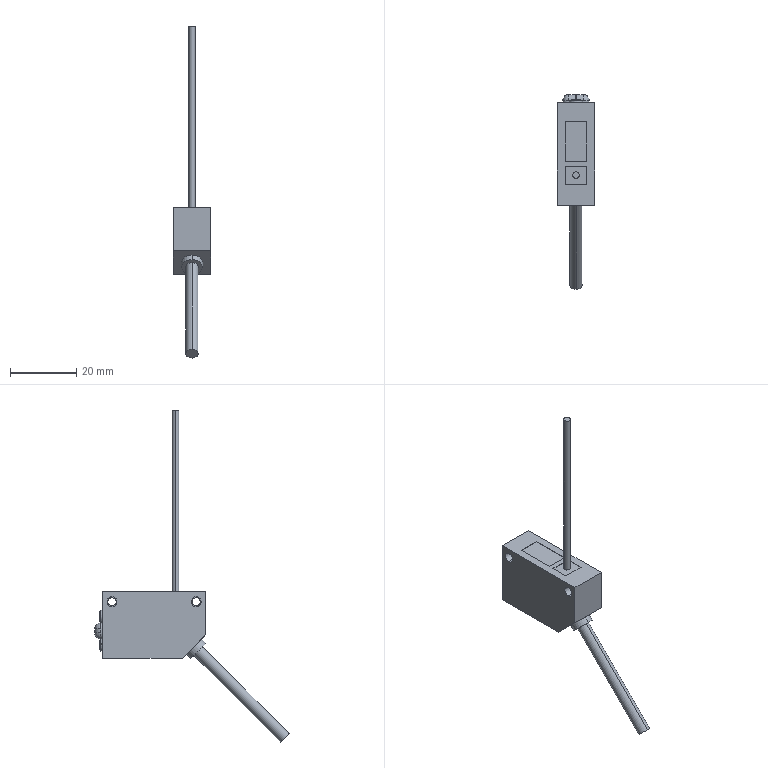Part | STEP file | Compact photoelectric sensor CX-441 | 3 solids | 95 faces | box 11.2 x 58.715 x 100.215 mm | volume 7246 mm3 | plane 50 | cylinder 34 | cone 7 | sphere 4 | commonest cylinder face diameters 3.6 x10 3 x8 2.5 x4 2.92 x4 2 x2 3.4 x2